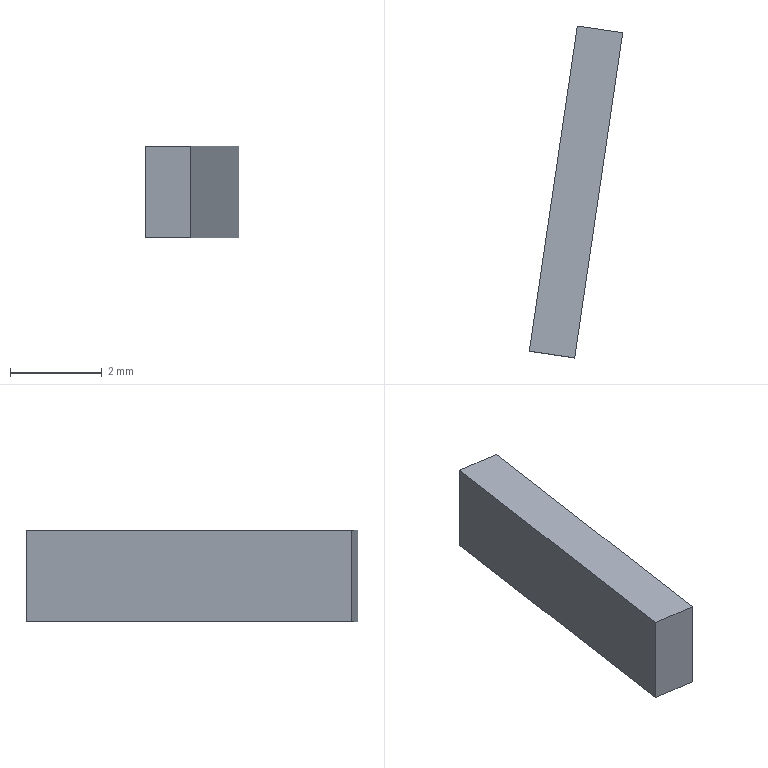Part | SolidWorks | features SplitBody 1 | 1 solid | 6 faces | box 2.034 x 7.221 x 2 mm | volume 14.304 mm3 | plane 6
STEP:
#1=CARTESIAN_POINT('',(71.726,4.807,-44.89));
#2=VERTEX_POINT('',#1);
#3=CARTESIAN_POINT('',(70.737,4.954,-44.89));
#4=VERTEX_POINT('',#3);
#5=CARTESIAN_POINT('',(71.726,4.807,-44.89));
#6=DIRECTION('',(-0.9893,0.1461,0.));
#7=VECTOR('',#6,1000.);
#8=LINE('',#5,#7);
#9=EDGE_CURVE('',#2,#4,#8,.T.);
#10=ORIENTED_EDGE('',*,*,#9,.F.);
#11=CARTESIAN_POINT('',(71.726,4.807,-42.89));
#12=VERTEX_POINT('',#11);
#13=CARTESIAN_POINT('',(71.726,4.807,-42.89));
#14=DIRECTION('',(0.,0.,-1.));
#15=VECTOR('',#14,1000.);
#16=LINE('',#13,#15);
#17=EDGE_CURVE('',#12,#2,#16,.T.);
#18=ORIENTED_EDGE('',*,*,#17,.F.);
#19=CARTESIAN_POINT('',(70.737,4.954,-42.89));
#20=VERTEX_POINT('',#19);
#21=CARTESIAN_POINT('',(71.726,4.807,-42.89));
#22=DIRECTION('',(-0.9893,0.1461,0.));
#23=VECTOR('',#22,1000.);
#24=LINE('',#21,#23);
#25=EDGE_CURVE('',#12,#20,#24,.T.);
#26=ORIENTED_EDGE('',*,*,#25,.T.);
#27=CARTESIAN_POINT('',(70.737,4.954,-42.89));
#28=DIRECTION('',(0.,0.,-1.));
#29=VECTOR('',#28,1000.);
#30=LINE('',#27,#29);
#31=EDGE_CURVE('',#20,#4,#30,.T.);
#32=ORIENTED_EDGE('',*,*,#31,.T.);
#33=EDGE_LOOP('',(#10,#18,#26,#32));
#34=FACE_OUTER_BOUND('',#33,.T.);
#35=CARTESIAN_POINT('',(71.726,4.807,-42.89));
#36=DIRECTION('',(-0.1461,-0.9893,0.));
#37=DIRECTION('',(0.9893,-0.1461,0.));
#38=AXIS2_PLACEMENT_3D('',#35,#36,#37);
#39=PLANE('',#38);
#40=ADVANCED_FACE('',(#34),#39,.T.);
#41=CARTESIAN_POINT('',(72.771,11.882,-44.89));
#42=VERTEX_POINT('',#41);
#43=CARTESIAN_POINT('',(72.771,11.882,-44.89));
#44=DIRECTION('',(-0.1461,-0.9893,0.));
#45=VECTOR('',#44,1000.);
#46=LINE('',#43,#45);
#47=EDGE_CURVE('',#42,#2,#46,.T.);
#48=ORIENTED_EDGE('',*,*,#47,.F.);
#49=CARTESIAN_POINT('',(72.771,11.882,-42.89));
#50=VERTEX_POINT('',#49);
#51=CARTESIAN_POINT('',(72.771,11.882,-42.89));
#52=DIRECTION('',(0.,0.,-1.));
#53=VECTOR('',#52,1000.);
#54=LINE('',#51,#53);
#55=EDGE_CURVE('',#50,#42,#54,.T.);
#56=ORIENTED_EDGE('',*,*,#55,.F.);
#57=CARTESIAN_POINT('',(72.771,11.882,-42.89));
#58=DIRECTION('',(-0.1461,-0.9893,0.));
#59=VECTOR('',#58,1000.);
#60=LINE('',#57,#59);
#61=EDGE_CURVE('',#50,#12,#60,.T.);
#62=ORIENTED_EDGE('',*,*,#61,.T.);
#63=ORIENTED_EDGE('',*,*,#17,.T.);
#64=EDGE_LOOP('',(#48,#56,#62,#63));
#65=FACE_OUTER_BOUND('',#64,.T.);
#66=CARTESIAN_POINT('',(72.771,11.882,-42.89));
#67=DIRECTION('',(0.9893,-0.1461,0.));
#68=DIRECTION('',(0.1461,0.9893,0.));
#69=AXIS2_PLACEMENT_3D('',#66,#67,#68);
#70=PLANE('',#69);
#71=ADVANCED_FACE('',(#65),#70,.T.);
#72=CARTESIAN_POINT('',(71.782,12.029,-44.89));
#73=VERTEX_POINT('',#72);
#74=CARTESIAN_POINT('',(71.782,12.029,-44.89));
#75=DIRECTION('',(0.9893,-0.1461,0.));
#76=VECTOR('',#75,1000.);
#77=LINE('',#74,#76);
#78=EDGE_CURVE('',#73,#42,#77,.T.);
#79=ORIENTED_EDGE('',*,*,#78,.F.);
#80=CARTESIAN_POINT('',(71.782,12.029,-42.89));
#81=VERTEX_POINT('',#80);
#82=CARTESIAN_POINT('',(71.782,12.029,-42.89));
#83=DIRECTION('',(0.,0.,-1.));
#84=VECTOR('',#83,1000.);
#85=LINE('',#82,#84);
#86=EDGE_CURVE('',#81,#73,#85,.T.);
#87=ORIENTED_EDGE('',*,*,#86,.F.);
#88=CARTESIAN_POINT('',(71.782,12.029,-42.89));
#89=DIRECTION('',(0.9893,-0.1461,0.));
#90=VECTOR('',#89,1000.);
#91=LINE('',#88,#90);
#92=EDGE_CURVE('',#81,#50,#91,.T.);
#93=ORIENTED_EDGE('',*,*,#92,.T.);
#94=ORIENTED_EDGE('',*,*,#55,.T.);
#95=EDGE_LOOP('',(#79,#87,#93,#94));
#96=FACE_OUTER_BOUND('',#95,.T.);
#97=CARTESIAN_POINT('',(71.782,12.029,-42.89));
#98=DIRECTION('',(0.1461,0.9893,0.));
#99=DIRECTION('',(-0.9893,0.1461,0.));
#100=AXIS2_PLACEMENT_3D('',#97,#98,#99);
#101=PLANE('',#100);
#102=ADVANCED_FACE('',(#96),#101,.T.);
#103=CARTESIAN_POINT('',(70.737,4.954,-44.89));
#104=DIRECTION('',(0.1461,0.9893,0.));
#105=VECTOR('',#104,1000.);
#106=LINE('',#103,#105);
#107=EDGE_CURVE('',#4,#73,#106,.T.);
#108=ORIENTED_EDGE('',*,*,#107,.F.);
#109=ORIENTED_EDGE('',*,*,#31,.F.);
#110=CARTESIAN_POINT('',(70.737,4.954,-42.89));
#111=DIRECTION('',(0.1461,0.9893,0.));
#112=VECTOR('',#111,1000.);
#113=LINE('',#110,#112);
#114=EDGE_CURVE('',#20,#81,#113,.T.);
#115=ORIENTED_EDGE('',*,*,#114,.T.);
#116=ORIENTED_EDGE('',*,*,#86,.T.);
#117=EDGE_LOOP('',(#108,#109,#115,#116));
#118=FACE_OUTER_BOUND('',#117,.T.);
#119=CARTESIAN_POINT('',(70.737,4.954,-42.89));
#120=DIRECTION('',(-0.9893,0.1461,0.));
#121=DIRECTION('',(-0.1461,-0.9893,0.));
#122=AXIS2_PLACEMENT_3D('',#119,#120,#121);
#123=PLANE('',#122);
#124=ADVANCED_FACE('',(#118),#123,.T.);
#125=ORIENTED_EDGE('',*,*,#25,.F.);
#126=ORIENTED_EDGE('',*,*,#61,.F.);
#127=ORIENTED_EDGE('',*,*,#92,.F.);
#128=ORIENTED_EDGE('',*,*,#114,.F.);
#129=EDGE_LOOP('',(#125,#126,#127,#128));
#130=FACE_OUTER_BOUND('',#129,.T.);
#131=CARTESIAN_POINT('',(0.,0.,-42.89));
#132=DIRECTION('',(0.,0.,-1.));
#133=DIRECTION('',(-1.,0.,0.));
#134=AXIS2_PLACEMENT_3D('',#131,#132,#133);
#135=PLANE('',#134);
#136=ADVANCED_FACE('',(#130),#135,.F.);
#137=ORIENTED_EDGE('',*,*,#9,.T.);
#138=ORIENTED_EDGE('',*,*,#107,.T.);
#139=ORIENTED_EDGE('',*,*,#78,.T.);
#140=ORIENTED_EDGE('',*,*,#47,.T.);
#141=EDGE_LOOP('',(#137,#138,#139,#140));
#142=FACE_OUTER_BOUND('',#141,.T.);
#143=CARTESIAN_POINT('',(0.,0.,-44.89));
#144=DIRECTION('',(0.,0.,-1.));
#145=DIRECTION('',(-1.,0.,0.));
#146=AXIS2_PLACEMENT_3D('',#143,#144,#145);
#147=PLANE('',#146);
#148=ADVANCED_FACE('',(#142),#147,.T.);
#149=CLOSED_SHELL('',(#40,#71,#102,#124,#136,#148));
#150=MANIFOLD_SOLID_BREP('',#149);
#151=CARTESIAN_POINT('',(0.,0.,0.));
#152=DIRECTION('',(0.,0.,1.));
#153=DIRECTION('',(1.,0.,0.));
#154=AXIS2_PLACEMENT_3D('',#151,#152,#153);
#155=(LENGTH_UNIT()NAMED_UNIT(*)SI_UNIT(.MILLI.,.METRE.));
#156=UNCERTAINTY_MEASURE_WITH_UNIT(LENGTH_MEASURE(0.00001),#155,'','');
#157=(NAMED_UNIT(*)PLANE_ANGLE_UNIT()SI_UNIT($,.RADIAN.));
#158=(NAMED_UNIT(*)SI_UNIT($,.STERADIAN.)SOLID_ANGLE_UNIT());
#159=(GEOMETRIC_REPRESENTATION_CONTEXT(3)GLOBAL_UNCERTAINTY_ASSIGNED_CONTEXT((#156))GLOBAL_UNIT_ASSIGNED_CONTEXT((#155,#157,#158))REPRESENTATION_CONTEXT('',''));
#160=ADVANCED_BREP_SHAPE_REPRESENTATION('',(#150,#154),#159);